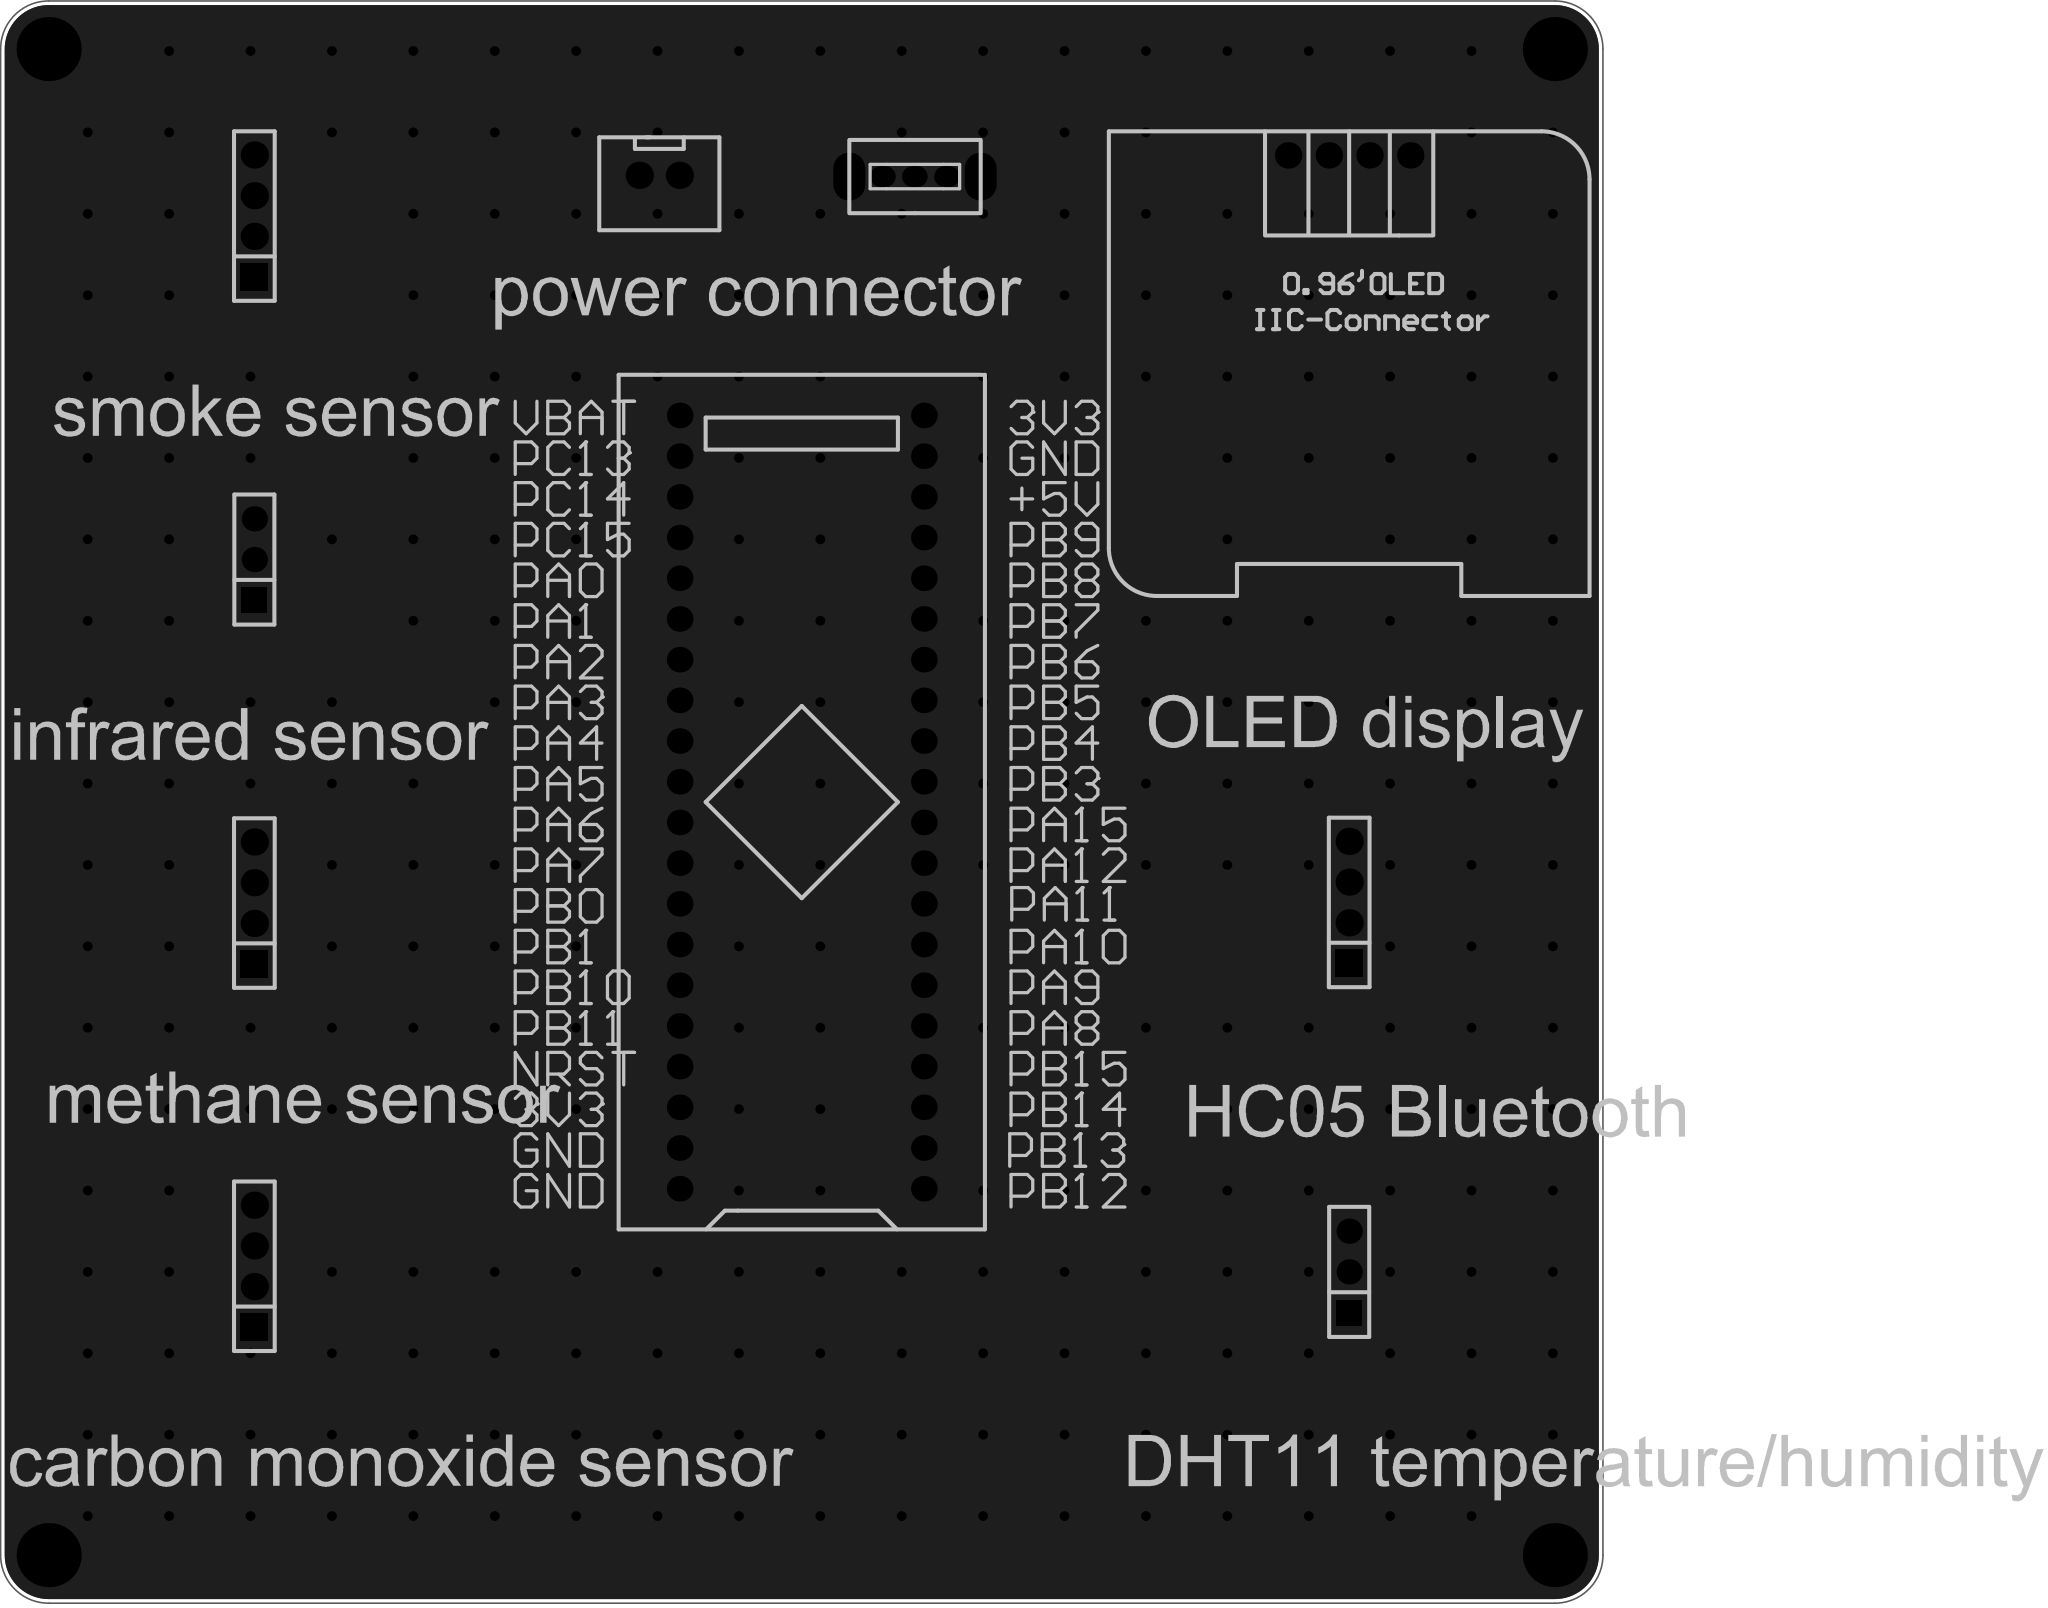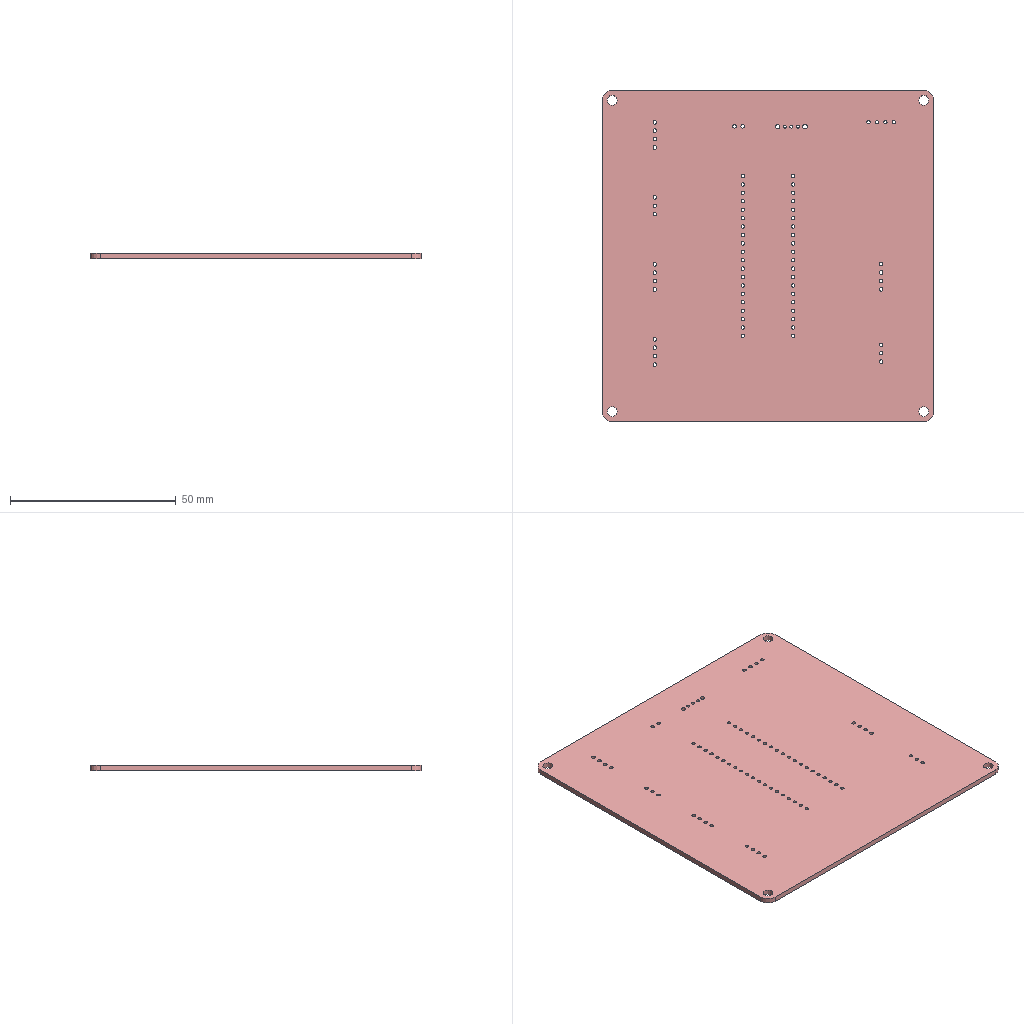Circuit board layout | Altium Designer | box 100 x 100 x 1.6 mm
Layer stack:
# Altium Designer layer stack of  (unit mm; dielectric type: 0 none, 1 core, 2 prepreg, 3 surface material)
index,name,kind,layer,copper_thickness_mm,dielectric_type,dielectric_thickness_mm,dielectric_material,dielectric_constant
0,Top Paste Mask Layer,other,,,,,,
1,Top Silkscreen Layer,other,,,,,,
2,Top Solder Mask Layer,dielectric,,,3,0.01,,3.3
3,Top Layer,copper,Top Layer,0.035,,,,
4,Dielectric1,dielectric,,,3,1.51,FR4,4.5
5,Bottom Layer,copper,Bottom Layer,0.035,,,,
6,Bottom Solder Mask Layer,dielectric,,,3,0.01,,3.3
7,Bottom Silkscreen Layer,other,,,,,,
8,Bottom Paste Mask Layer,other,,,,,,
# drill layer pairs: low layer,high layer
drill_pair,Top Layer,Bottom Layer
Part placement:
Designator,Comment,Layer,Footprint,Center-X(mm),Center-Y(mm),Rotation
U1,STM32F103C8T6-Card,TopLayer,CONN-TH_L53.3-W22.9_STM32F103C8T6-CARD,141.351,130.937,90
OLED1,,TopLayer,0.96OLED_4P,175.514,171.301,0
CN4,XH2.54*2P_through-hole,TopLayer,CONN-TH_2P-P2.50-XH2.54-2P,132.461,170.053,0
SW5,,TopLayer,拨动开关,148.417,169.978,0
H1,,TopLayer,HDR-TH_3P-P2.54-V-F,107.188,146.074,90
H2,,TopLayer,HDR-TH_4P-P2.54-V-F,175.514,124.674,90
H3,,TopLayer,HDR-TH_3P-P2.54-V-F,175.514,101.615,90
H4,,TopLayer,HDR-TH_4P-P2.54-V-F,107.188,167.513,90
H5,,TopLayer,HDR-TH_4P-P2.54-V-F,107.188,124.636,90
H6,,TopLayer,HDR-TH_4P-P2.54-V-F,107.188,101.967,90
Pad and via stacks:
# Altium Designer via and pad stacks of  (unit mm). Each distinct definition once, with the count of objects using it.
# via: kind,start_layer,end_layer,hole_mm,diameter_mm,mode(0 simple;1 top-mid-bottom;2 full stack),diameter_per_layer,count,example_net
# pad: kind,layer,hole_mm,hole_type(0 round;1 square;2 slot),plating,top_size,top_shape(1 round;2 rect;3 octagon;9 rounded rect),mid_size,bottom_size,mode,footprint,size_per_layer,count,example
pad,Multi-Layer,3,0,plated,4x4,1,4x4,4x4,0,,,4,1
pad,Multi-Layer,1,0,plated,1.6x1.6,1,1.6x1.6,1.6x1.6,0,CONN-TH_L53.3-W22.9_STM32F103C8T6-CARD,,40,U1.1
pad,Multi-Layer,1,0,plated,1.65x1.65,1,1.65x1.65,1.65x1.65,0,0.96OLED_4P,,4,OLED1.4
pad,Multi-Layer,1.05,0,plated,1.7x1.7,1,1.7x1.7,1.7x1.7,0,CONN-TH_2P-P2.50-XH2.54-2P,,2,CN4.2
pad,Multi-Layer,0.8992,0,plated,1.6x1.3,1,1.6x1.3,1.6x1.3,0,\u00B2\u00A6\u00B6\u00AF\u00BF\u00AA\u00B9\u00D8,,3,SW5.1
pad,Multi-Layer,1.3,0,plated,3x1.999,1,3x1.999,3x1.999,0,\u00B2\u00A6\u00B6\u00AF\u00BF\u00AA\u00B9\u00D8,,2,SW5.4
pad,Multi-Layer,1.02,0,plated,1.575x1.575,1,1.575x1.575,1.575x1.575,0,HDR-TH_3P-P2.54-V-F,,4,H1.3
pad,Multi-Layer,1.02,0,plated,1.575x1.575,2,1.575x1.575,1.575x1.575,0,HDR-TH_3P-P2.54-V-F,,2,H1.1
pad,Multi-Layer,1.1,0,plated,1.7x1.7,2,1.7x1.7,1.7x1.7,0,HDR-TH_4P-P2.54-V-F,,4,H2.1
pad,Multi-Layer,1.1,0,plated,1.7x1.7,1,1.7x1.7,1.7x1.7,0,HDR-TH_4P-P2.54-V-F,,12,H2.2
via,Top Layer,Bottom Layer,0.3048,0.61,0,,297,GND
Copper pours:
name,layer,net,type(0 solid;1 hatched;2 none)
Bottom Layer-GND,Bottom Layer,GND,0
Top Layer-GND,Top Layer,GND,0